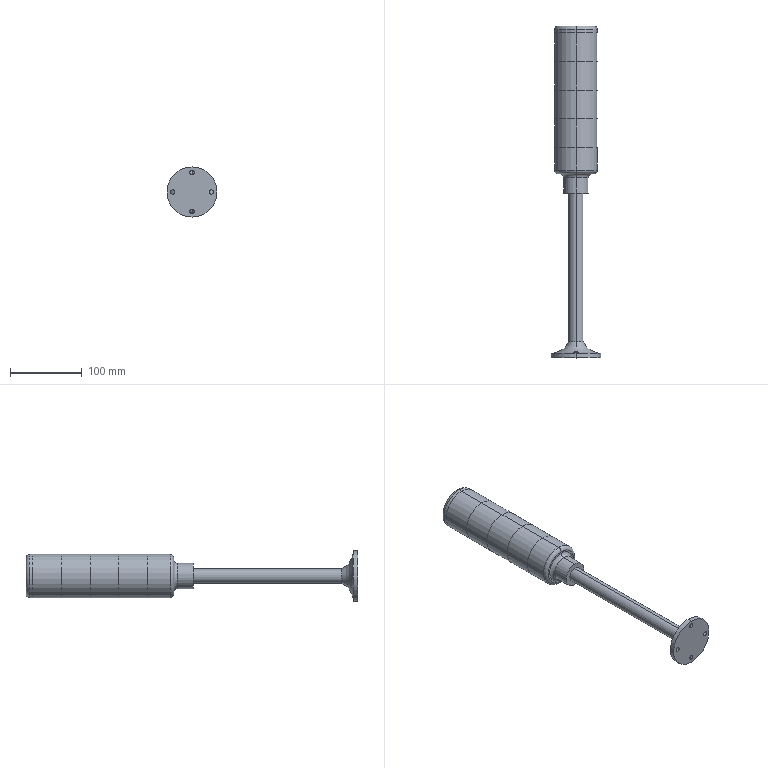Part | SolidWorks | features ICE 9, Fillet 3, Extrusion 1, HoleWzd 1, RevCut 1 | 6 solids | 48 faces | box 70 x 462.6 x 70 mm | volume 712643 mm3 | cylinder 26 | plane 14 | torus 8 | commonest cylinder face diameters 60 x12 6 x8 20 x2 35 x2 70 x2